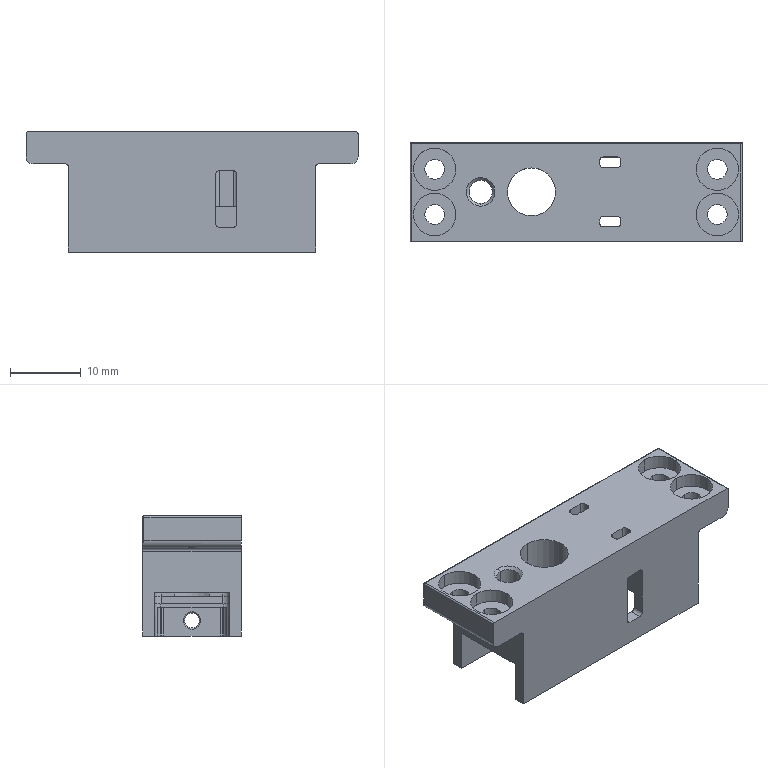Part | 1 solid | 128 faces | box 47 x 14 x 17 mm | volume 5977 mm3 | cylinder 72 | plane 47 | cone 8 | sphere 1 | commonest cylinder face diameters 1 x20 1.6 x9 2 x8 2.8 x8 6 x8 0.4 x4